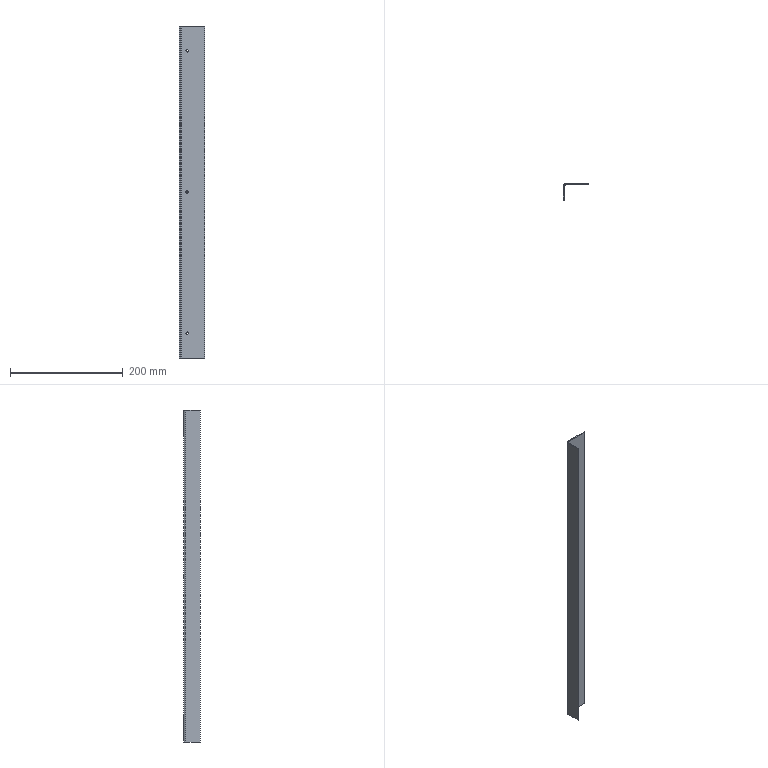Part | STEP file | SYL_0392D6J1SYL0380DJ10-1725835 | 1 solid | 20 faces | box 44.9 x 29.9 x 588 mm | volume 79950 mm3 | plane 12 | cylinder 8 | commonest cylinder face diameters 4.2 x6 4 x1 7.8 x1
STEP:
#1=CARTESIAN_POINT('',(-8.5,29.9,-247.9));
#2=VERTEX_POINT('',#1);
#3=CARTESIAN_POINT('',(-8.5,28.,-247.9));
#4=VERTEX_POINT('',#3);
#5=CARTESIAN_POINT('',(-8.5,28.,-247.9));
#6=DIRECTION('',(0.,-1.,0.));
#7=VECTOR('',#6,1000.);
#8=LINE('',#5,#7);
#9=EDGE_CURVE('',#2,#4,#8,.T.);
#10=ORIENTED_EDGE('',*,*,#9,.F.);
#11=CARTESIAN_POINT('',(-8.5,29.9,-252.1));
#12=VERTEX_POINT('',#11);
#13=CARTESIAN_POINT('',(-8.5,29.9,-250.));
#14=DIRECTION('',(0.,1.,0.));
#15=DIRECTION('',(0.,0.,1.));
#16=AXIS2_PLACEMENT_3D('',#13,#14,#15);
#17=CIRCLE('',#16,2.1);
#18=EDGE_CURVE('',#2,#12,#17,.T.);
#19=ORIENTED_EDGE('',*,*,#18,.T.);
#20=CARTESIAN_POINT('',(-8.5,28.,-252.1));
#21=VERTEX_POINT('',#20);
#22=CARTESIAN_POINT('',(-8.5,28.,-252.1));
#23=DIRECTION('',(0.,-1.,0.));
#24=VECTOR('',#23,1000.);
#25=LINE('',#22,#24);
#26=EDGE_CURVE('',#12,#21,#25,.T.);
#27=ORIENTED_EDGE('',*,*,#26,.T.);
#28=CARTESIAN_POINT('',(-8.5,28.,-250.));
#29=DIRECTION('',(0.,1.,0.));
#30=DIRECTION('',(0.,0.,1.));
#31=AXIS2_PLACEMENT_3D('',#28,#29,#30);
#32=CIRCLE('',#31,2.1);
#33=EDGE_CURVE('',#4,#21,#32,.T.);
#34=ORIENTED_EDGE('',*,*,#33,.F.);
#35=EDGE_LOOP('',(#10,#19,#27,#34));
#36=FACE_OUTER_BOUND('',#35,.T.);
#37=CARTESIAN_POINT('',(-8.5,28.,-250.));
#38=DIRECTION('',(0.,1.,0.));
#39=DIRECTION('',(0.,0.,1.));
#40=AXIS2_PLACEMENT_3D('',#37,#38,#39);
#41=CYLINDRICAL_SURFACE('',#40,2.1);
#42=ADVANCED_FACE('',(#36),#41,.F.);
#43=CARTESIAN_POINT('',(-8.5,29.9,2.1));
#44=VERTEX_POINT('',#43);
#45=CARTESIAN_POINT('',(-8.5,28.,2.1));
#46=VERTEX_POINT('',#45);
#47=CARTESIAN_POINT('',(-8.5,28.,2.1));
#48=DIRECTION('',(0.,-1.,0.));
#49=VECTOR('',#48,1000.);
#50=LINE('',#47,#49);
#51=EDGE_CURVE('',#44,#46,#50,.T.);
#52=ORIENTED_EDGE('',*,*,#51,.F.);
#53=CARTESIAN_POINT('',(-8.5,29.9,-2.1));
#54=VERTEX_POINT('',#53);
#55=CARTESIAN_POINT('',(-8.5,29.9,0.));
#56=DIRECTION('',(0.,1.,0.));
#57=DIRECTION('',(0.,0.,1.));
#58=AXIS2_PLACEMENT_3D('',#55,#56,#57);
#59=CIRCLE('',#58,2.1);
#60=EDGE_CURVE('',#44,#54,#59,.T.);
#61=ORIENTED_EDGE('',*,*,#60,.T.);
#62=CARTESIAN_POINT('',(-8.5,28.,-2.1));
#63=VERTEX_POINT('',#62);
#64=CARTESIAN_POINT('',(-8.5,28.,-2.1));
#65=DIRECTION('',(0.,-1.,0.));
#66=VECTOR('',#65,1000.);
#67=LINE('',#64,#66);
#68=EDGE_CURVE('',#54,#63,#67,.T.);
#69=ORIENTED_EDGE('',*,*,#68,.T.);
#70=CARTESIAN_POINT('',(-8.5,28.,0.));
#71=DIRECTION('',(0.,1.,0.));
#72=DIRECTION('',(0.,0.,1.));
#73=AXIS2_PLACEMENT_3D('',#70,#71,#72);
#74=CIRCLE('',#73,2.1);
#75=EDGE_CURVE('',#46,#63,#74,.T.);
#76=ORIENTED_EDGE('',*,*,#75,.F.);
#77=EDGE_LOOP('',(#52,#61,#69,#76));
#78=FACE_OUTER_BOUND('',#77,.T.);
#79=CARTESIAN_POINT('',(-8.5,28.,0.));
#80=DIRECTION('',(0.,1.,0.));
#81=DIRECTION('',(0.,0.,1.));
#82=AXIS2_PLACEMENT_3D('',#79,#80,#81);
#83=CYLINDRICAL_SURFACE('',#82,2.1);
#84=ADVANCED_FACE('',(#78),#83,.F.);
#85=CARTESIAN_POINT('',(-8.5,29.9,252.1));
#86=VERTEX_POINT('',#85);
#87=CARTESIAN_POINT('',(-8.5,28.,252.1));
#88=VERTEX_POINT('',#87);
#89=CARTESIAN_POINT('',(-8.5,28.,252.1));
#90=DIRECTION('',(0.,-1.,0.));
#91=VECTOR('',#90,1000.);
#92=LINE('',#89,#91);
#93=EDGE_CURVE('',#86,#88,#92,.T.);
#94=ORIENTED_EDGE('',*,*,#93,.F.);
#95=CARTESIAN_POINT('',(-8.5,29.9,247.9));
#96=VERTEX_POINT('',#95);
#97=CARTESIAN_POINT('',(-8.5,29.9,250.));
#98=DIRECTION('',(0.,1.,0.));
#99=DIRECTION('',(0.,0.,1.));
#100=AXIS2_PLACEMENT_3D('',#97,#98,#99);
#101=CIRCLE('',#100,2.1);
#102=EDGE_CURVE('',#86,#96,#101,.T.);
#103=ORIENTED_EDGE('',*,*,#102,.T.);
#104=CARTESIAN_POINT('',(-8.5,28.,247.9));
#105=VERTEX_POINT('',#104);
#106=CARTESIAN_POINT('',(-8.5,28.,247.9));
#107=DIRECTION('',(0.,-1.,0.));
#108=VECTOR('',#107,1000.);
#109=LINE('',#106,#108);
#110=EDGE_CURVE('',#96,#105,#109,.T.);
#111=ORIENTED_EDGE('',*,*,#110,.T.);
#112=CARTESIAN_POINT('',(-8.5,28.,250.));
#113=DIRECTION('',(0.,1.,0.));
#114=DIRECTION('',(0.,0.,1.));
#115=AXIS2_PLACEMENT_3D('',#112,#113,#114);
#116=CIRCLE('',#115,2.1);
#117=EDGE_CURVE('',#88,#105,#116,.T.);
#118=ORIENTED_EDGE('',*,*,#117,.F.);
#119=EDGE_LOOP('',(#94,#103,#111,#118));
#120=FACE_OUTER_BOUND('',#119,.T.);
#121=CARTESIAN_POINT('',(-8.5,28.,250.));
#122=DIRECTION('',(0.,1.,0.));
#123=DIRECTION('',(0.,0.,1.));
#124=AXIS2_PLACEMENT_3D('',#121,#122,#123);
#125=CYLINDRICAL_SURFACE('',#124,2.1);
#126=ADVANCED_FACE('',(#120),#125,.F.);
#127=CARTESIAN_POINT('',(-22.4,0.,294.));
#128=VERTEX_POINT('',#127);
#129=CARTESIAN_POINT('',(-20.5,0.,294.));
#130=VERTEX_POINT('',#129);
#131=CARTESIAN_POINT('',(-20.5,0.,294.));
#132=DIRECTION('',(1.,0.,0.));
#133=VECTOR('',#132,1000.);
#134=LINE('',#131,#133);
#135=EDGE_CURVE('',#128,#130,#134,.T.);
#136=ORIENTED_EDGE('',*,*,#135,.F.);
#137=CARTESIAN_POINT('',(-22.4,0.,-294.));
#138=VERTEX_POINT('',#137);
#139=CARTESIAN_POINT('',(-22.4,0.,-294.));
#140=DIRECTION('',(0.,0.,-1.));
#141=VECTOR('',#140,1000.);
#142=LINE('',#139,#141);
#143=EDGE_CURVE('',#128,#138,#142,.T.);
#144=ORIENTED_EDGE('',*,*,#143,.T.);
#145=CARTESIAN_POINT('',(-20.5,0.,-294.));
#146=VERTEX_POINT('',#145);
#147=CARTESIAN_POINT('',(-20.5,0.,-294.));
#148=DIRECTION('',(1.,0.,0.));
#149=VECTOR('',#148,1000.);
#150=LINE('',#147,#149);
#151=EDGE_CURVE('',#138,#146,#150,.T.);
#152=ORIENTED_EDGE('',*,*,#151,.T.);
#153=CARTESIAN_POINT('',(-20.5,0.,294.));
#154=DIRECTION('',(0.,0.,-1.));
#155=VECTOR('',#154,1000.);
#156=LINE('',#153,#155);
#157=EDGE_CURVE('',#130,#146,#156,.T.);
#158=ORIENTED_EDGE('',*,*,#157,.F.);
#159=EDGE_LOOP('',(#136,#144,#152,#158));
#160=FACE_OUTER_BOUND('',#159,.T.);
#161=CARTESIAN_POINT('',(-20.5,0.,294.));
#162=DIRECTION('',(0.,1.,0.));
#163=DIRECTION('',(0.,0.,-1.));
#164=AXIS2_PLACEMENT_3D('',#161,#162,#163);
#165=PLANE('',#164);
#166=ADVANCED_FACE('',(#160),#165,.F.);
#167=ORIENTED_EDGE('',*,*,#151,.F.);
#168=CARTESIAN_POINT('',(-22.4,26.,-294.));
#169=VERTEX_POINT('',#168);
#170=CARTESIAN_POINT('',(-22.4,30.,-294.));
#171=DIRECTION('',(0.,1.,0.));
#172=VECTOR('',#171,1000.);
#173=LINE('',#170,#172);
#174=EDGE_CURVE('',#138,#169,#173,.T.);
#175=ORIENTED_EDGE('',*,*,#174,.T.);
#176=CARTESIAN_POINT('',(-20.5,26.,-294.));
#177=VERTEX_POINT('',#176);
#178=CARTESIAN_POINT('',(-20.5,26.,-294.));
#179=DIRECTION('',(1.,0.,0.));
#180=VECTOR('',#179,1000.);
#181=LINE('',#178,#180);
#182=EDGE_CURVE('',#169,#177,#181,.T.);
#183=ORIENTED_EDGE('',*,*,#182,.T.);
#184=CARTESIAN_POINT('',(-20.5,0.,-294.));
#185=DIRECTION('',(0.,1.,0.));
#186=VECTOR('',#185,1000.);
#187=LINE('',#184,#186);
#188=EDGE_CURVE('',#146,#177,#187,.T.);
#189=ORIENTED_EDGE('',*,*,#188,.F.);
#190=EDGE_LOOP('',(#167,#175,#183,#189));
#191=FACE_OUTER_BOUND('',#190,.T.);
#192=CARTESIAN_POINT('',(-20.5,0.,-294.));
#193=DIRECTION('',(0.,0.,1.));
#194=DIRECTION('',(0.,1.,0.));
#195=AXIS2_PLACEMENT_3D('',#192,#193,#194);
#196=PLANE('',#195);
#197=ADVANCED_FACE('',(#191),#196,.F.);
#198=ORIENTED_EDGE('',*,*,#182,.F.);
#199=CARTESIAN_POINT('',(-18.5,29.9,-294.));
#200=VERTEX_POINT('',#199);
#201=CARTESIAN_POINT('',(-18.5,26.,-294.));
#202=DIRECTION('',(0.,0.,1.));
#203=DIRECTION('',(-1.,0.,0.));
#204=AXIS2_PLACEMENT_3D('',#201,#202,#203);
#205=CIRCLE('',#204,3.9);
#206=EDGE_CURVE('',#200,#169,#205,.T.);
#207=ORIENTED_EDGE('',*,*,#206,.F.);
#208=CARTESIAN_POINT('',(-18.5,28.,-294.));
#209=VERTEX_POINT('',#208);
#210=CARTESIAN_POINT('',(-18.5,28.,-294.));
#211=DIRECTION('',(0.,-1.,0.));
#212=VECTOR('',#211,1000.);
#213=LINE('',#210,#212);
#214=EDGE_CURVE('',#200,#209,#213,.T.);
#215=ORIENTED_EDGE('',*,*,#214,.T.);
#216=CARTESIAN_POINT('',(-18.5,26.,-294.));
#217=DIRECTION('',(0.,0.,1.));
#218=DIRECTION('',(0.,1.,0.));
#219=AXIS2_PLACEMENT_3D('',#216,#217,#218);
#220=CIRCLE('',#219,2.);
#221=EDGE_CURVE('',#209,#177,#220,.T.);
#222=ORIENTED_EDGE('',*,*,#221,.T.);
#223=EDGE_LOOP('',(#198,#207,#215,#222));
#224=FACE_OUTER_BOUND('',#223,.T.);
#225=CARTESIAN_POINT('',(-18.5,26.,-294.));
#226=DIRECTION('',(0.,0.,-1.));
#227=DIRECTION('',(-1.,0.,0.));
#228=AXIS2_PLACEMENT_3D('',#225,#226,#227);
#229=PLANE('',#228);
#230=ADVANCED_FACE('',(#224),#229,.T.);
#231=ORIENTED_EDGE('',*,*,#214,.F.);
#232=CARTESIAN_POINT('',(22.5,29.9,-294.));
#233=VERTEX_POINT('',#232);
#234=CARTESIAN_POINT('',(22.5,29.9,-294.));
#235=DIRECTION('',(1.,0.,0.));
#236=VECTOR('',#235,1000.);
#237=LINE('',#234,#236);
#238=EDGE_CURVE('',#200,#233,#237,.T.);
#239=ORIENTED_EDGE('',*,*,#238,.T.);
#240=CARTESIAN_POINT('',(22.5,28.,-294.));
#241=VERTEX_POINT('',#240);
#242=CARTESIAN_POINT('',(22.5,28.,-294.));
#243=DIRECTION('',(0.,-1.,0.));
#244=VECTOR('',#243,1000.);
#245=LINE('',#242,#244);
#246=EDGE_CURVE('',#233,#241,#245,.T.);
#247=ORIENTED_EDGE('',*,*,#246,.T.);
#248=CARTESIAN_POINT('',(-18.5,28.,-294.));
#249=DIRECTION('',(1.,0.,0.));
#250=VECTOR('',#249,1000.);
#251=LINE('',#248,#250);
#252=EDGE_CURVE('',#209,#241,#251,.T.);
#253=ORIENTED_EDGE('',*,*,#252,.F.);
#254=EDGE_LOOP('',(#231,#239,#247,#253));
#255=FACE_OUTER_BOUND('',#254,.T.);
#256=CARTESIAN_POINT('',(-18.5,28.,-294.));
#257=DIRECTION('',(0.,0.,1.));
#258=DIRECTION('',(1.,0.,0.));
#259=AXIS2_PLACEMENT_3D('',#256,#257,#258);
#260=PLANE('',#259);
#261=ADVANCED_FACE('',(#255),#260,.F.);
#262=ORIENTED_EDGE('',*,*,#246,.F.);
#263=CARTESIAN_POINT('',(22.5,29.9,294.));
#264=VERTEX_POINT('',#263);
#265=CARTESIAN_POINT('',(22.5,29.9,-294.));
#266=DIRECTION('',(0.,0.,1.));
#267=VECTOR('',#266,1000.);
#268=LINE('',#265,#267);
#269=EDGE_CURVE('',#233,#264,#268,.T.);
#270=ORIENTED_EDGE('',*,*,#269,.T.);
#271=CARTESIAN_POINT('',(22.5,28.,294.));
#272=VERTEX_POINT('',#271);
#273=CARTESIAN_POINT('',(22.5,28.,294.));
#274=DIRECTION('',(0.,-1.,0.));
#275=VECTOR('',#274,1000.);
#276=LINE('',#273,#275);
#277=EDGE_CURVE('',#264,#272,#276,.T.);
#278=ORIENTED_EDGE('',*,*,#277,.T.);
#279=CARTESIAN_POINT('',(22.5,28.,-294.));
#280=DIRECTION('',(0.,0.,1.));
#281=VECTOR('',#280,1000.);
#282=LINE('',#279,#281);
#283=EDGE_CURVE('',#241,#272,#282,.T.);
#284=ORIENTED_EDGE('',*,*,#283,.F.);
#285=EDGE_LOOP('',(#262,#270,#278,#284));
#286=FACE_OUTER_BOUND('',#285,.T.);
#287=CARTESIAN_POINT('',(22.5,28.,-294.));
#288=DIRECTION('',(-1.,0.,0.));
#289=DIRECTION('',(0.,0.,1.));
#290=AXIS2_PLACEMENT_3D('',#287,#288,#289);
#291=PLANE('',#290);
#292=ADVANCED_FACE('',(#286),#291,.F.);
#293=ORIENTED_EDGE('',*,*,#277,.F.);
#294=CARTESIAN_POINT('',(-18.5,29.9,294.));
#295=VERTEX_POINT('',#294);
#296=CARTESIAN_POINT('',(22.5,29.9,294.));
#297=DIRECTION('',(-1.,0.,0.));
#298=VECTOR('',#297,1000.);
#299=LINE('',#296,#298);
#300=EDGE_CURVE('',#264,#295,#299,.T.);
#301=ORIENTED_EDGE('',*,*,#300,.T.);
#302=CARTESIAN_POINT('',(-18.5,28.,294.));
#303=VERTEX_POINT('',#302);
#304=CARTESIAN_POINT('',(-18.5,28.,294.));
#305=DIRECTION('',(0.,-1.,0.));
#306=VECTOR('',#305,1000.);
#307=LINE('',#304,#306);
#308=EDGE_CURVE('',#295,#303,#307,.T.);
#309=ORIENTED_EDGE('',*,*,#308,.T.);
#310=CARTESIAN_POINT('',(22.5,28.,294.));
#311=DIRECTION('',(-1.,0.,0.));
#312=VECTOR('',#311,1000.);
#313=LINE('',#310,#312);
#314=EDGE_CURVE('',#272,#303,#313,.T.);
#315=ORIENTED_EDGE('',*,*,#314,.F.);
#316=EDGE_LOOP('',(#293,#301,#309,#315));
#317=FACE_OUTER_BOUND('',#316,.T.);
#318=CARTESIAN_POINT('',(22.5,28.,294.));
#319=DIRECTION('',(0.,0.,-1.));
#320=DIRECTION('',(-1.,0.,0.));
#321=AXIS2_PLACEMENT_3D('',#318,#319,#320);
#322=PLANE('',#321);
#323=ADVANCED_FACE('',(#317),#322,.F.);
#324=ORIENTED_EDGE('',*,*,#308,.F.);
#325=CARTESIAN_POINT('',(-22.4,26.,294.));
#326=VERTEX_POINT('',#325);
#327=CARTESIAN_POINT('',(-18.5,26.,294.));
#328=DIRECTION('',(0.,0.,-1.));
#329=DIRECTION('',(-1.,0.,0.));
#330=AXIS2_PLACEMENT_3D('',#327,#328,#329);
#331=CIRCLE('',#330,3.9);
#332=EDGE_CURVE('',#326,#295,#331,.T.);
#333=ORIENTED_EDGE('',*,*,#332,.F.);
#334=CARTESIAN_POINT('',(-20.5,26.,294.));
#335=VERTEX_POINT('',#334);
#336=CARTESIAN_POINT('',(-20.5,26.,294.));
#337=DIRECTION('',(1.,0.,0.));
#338=VECTOR('',#337,1000.);
#339=LINE('',#336,#338);
#340=EDGE_CURVE('',#326,#335,#339,.T.);
#341=ORIENTED_EDGE('',*,*,#340,.T.);
#342=CARTESIAN_POINT('',(-18.5,26.,294.));
#343=DIRECTION('',(0.,0.,-1.));
#344=DIRECTION('',(-1.,0.,0.));
#345=AXIS2_PLACEMENT_3D('',#342,#343,#344);
#346=CIRCLE('',#345,2.);
#347=EDGE_CURVE('',#335,#303,#346,.T.);
#348=ORIENTED_EDGE('',*,*,#347,.T.);
#349=EDGE_LOOP('',(#324,#333,#341,#348));
#350=FACE_OUTER_BOUND('',#349,.T.);
#351=CARTESIAN_POINT('',(-18.5,26.,294.));
#352=DIRECTION('',(0.,0.,1.));
#353=DIRECTION('',(1.,0.,0.));
#354=AXIS2_PLACEMENT_3D('',#351,#352,#353);
#355=PLANE('',#354);
#356=ADVANCED_FACE('',(#350),#355,.T.);
#357=CARTESIAN_POINT('',(-8.5,29.9,250.));
#358=DIRECTION('',(0.,1.,0.));
#359=DIRECTION('',(0.,0.,1.));
#360=AXIS2_PLACEMENT_3D('',#357,#358,#359);
#361=CIRCLE('',#360,2.1);
#362=EDGE_CURVE('',#96,#86,#361,.T.);
#363=ORIENTED_EDGE('',*,*,#362,.T.);
#364=ORIENTED_EDGE('',*,*,#93,.T.);
#365=CARTESIAN_POINT('',(-8.5,28.,250.));
#366=DIRECTION('',(0.,1.,0.));
#367=DIRECTION('',(0.,0.,-1.));
#368=AXIS2_PLACEMENT_3D('',#365,#366,#367);
#369=CIRCLE('',#368,2.1);
#370=EDGE_CURVE('',#105,#88,#369,.T.);
#371=ORIENTED_EDGE('',*,*,#370,.F.);
#372=ORIENTED_EDGE('',*,*,#110,.F.);
#373=EDGE_LOOP('',(#363,#364,#371,#372));
#374=FACE_OUTER_BOUND('',#373,.T.);
#375=CARTESIAN_POINT('',(-8.5,28.,250.));
#376=DIRECTION('',(0.,1.,0.));
#377=DIRECTION('',(0.,0.,1.));
#378=AXIS2_PLACEMENT_3D('',#375,#376,#377);
#379=CYLINDRICAL_SURFACE('',#378,2.1);
#380=ADVANCED_FACE('',(#374),#379,.F.);
#381=CARTESIAN_POINT('',(-8.5,29.9,0.));
#382=DIRECTION('',(0.,1.,0.));
#383=DIRECTION('',(0.,0.,1.));
#384=AXIS2_PLACEMENT_3D('',#381,#382,#383);
#385=CIRCLE('',#384,2.1);
#386=EDGE_CURVE('',#54,#44,#385,.T.);
#387=ORIENTED_EDGE('',*,*,#386,.T.);
#388=ORIENTED_EDGE('',*,*,#51,.T.);
#389=CARTESIAN_POINT('',(-8.5,28.,0.));
#390=DIRECTION('',(0.,1.,0.));
#391=DIRECTION('',(0.,0.,-1.));
#392=AXIS2_PLACEMENT_3D('',#389,#390,#391);
#393=CIRCLE('',#392,2.1);
#394=EDGE_CURVE('',#63,#46,#393,.T.);
#395=ORIENTED_EDGE('',*,*,#394,.F.);
#396=ORIENTED_EDGE('',*,*,#68,.F.);
#397=EDGE_LOOP('',(#387,#388,#395,#396));
#398=FACE_OUTER_BOUND('',#397,.T.);
#399=CARTESIAN_POINT('',(-8.5,28.,0.));
#400=DIRECTION('',(0.,1.,0.));
#401=DIRECTION('',(0.,0.,1.));
#402=AXIS2_PLACEMENT_3D('',#399,#400,#401);
#403=CYLINDRICAL_SURFACE('',#402,2.1);
#404=ADVANCED_FACE('',(#398),#403,.F.);
#405=CARTESIAN_POINT('',(-8.5,29.9,-250.));
#406=DIRECTION('',(0.,1.,0.));
#407=DIRECTION('',(0.,0.,1.));
#408=AXIS2_PLACEMENT_3D('',#405,#406,#407);
#409=CIRCLE('',#408,2.1);
#410=EDGE_CURVE('',#12,#2,#409,.T.);
#411=ORIENTED_EDGE('',*,*,#410,.T.);
#412=ORIENTED_EDGE('',*,*,#9,.T.);
#413=CARTESIAN_POINT('',(-8.5,28.,-250.));
#414=DIRECTION('',(0.,1.,0.));
#415=DIRECTION('',(0.,0.,-1.));
#416=AXIS2_PLACEMENT_3D('',#413,#414,#415);
#417=CIRCLE('',#416,2.1);
#418=EDGE_CURVE('',#21,#4,#417,.T.);
#419=ORIENTED_EDGE('',*,*,#418,.F.);
#420=ORIENTED_EDGE('',*,*,#26,.F.);
#421=EDGE_LOOP('',(#411,#412,#419,#420));
#422=FACE_OUTER_BOUND('',#421,.T.);
#423=CARTESIAN_POINT('',(-8.5,28.,-250.));
#424=DIRECTION('',(0.,1.,0.));
#425=DIRECTION('',(0.,0.,1.));
#426=AXIS2_PLACEMENT_3D('',#423,#424,#425);
#427=CYLINDRICAL_SURFACE('',#426,2.1);
#428=ADVANCED_FACE('',(#422),#427,.F.);
#429=CARTESIAN_POINT('',(-22.4,30.,294.));
#430=DIRECTION('',(0.,-1.,0.));
#431=VECTOR('',#430,1000.);
#432=LINE('',#429,#431);
#433=EDGE_CURVE('',#326,#128,#432,.T.);
#434=ORIENTED_EDGE('',*,*,#433,.T.);
#435=ORIENTED_EDGE('',*,*,#135,.T.);
#436=CARTESIAN_POINT('',(-20.5,26.,294.));
#437=DIRECTION('',(0.,-1.,0.));
#438=VECTOR('',#437,1000.);
#439=LINE('',#436,#438);
#440=EDGE_CURVE('',#335,#130,#439,.T.);
#441=ORIENTED_EDGE('',*,*,#440,.F.);
#442=ORIENTED_EDGE('',*,*,#340,.F.);
#443=EDGE_LOOP('',(#434,#435,#441,#442));
#444=FACE_OUTER_BOUND('',#443,.T.);
#445=CARTESIAN_POINT('',(-20.5,26.,294.));
#446=DIRECTION('',(0.,0.,-1.));
#447=DIRECTION('',(0.,-1.,0.));
#448=AXIS2_PLACEMENT_3D('',#445,#446,#447);
#449=PLANE('',#448);
#450=ADVANCED_FACE('',(#444),#449,.F.);
#451=ORIENTED_EDGE('',*,*,#347,.F.);
#452=CARTESIAN_POINT('',(-20.5,26.,294.));
#453=DIRECTION('',(0.,0.,-1.));
#454=VECTOR('',#453,1000.);
#455=LINE('',#452,#454);
#456=EDGE_CURVE('',#335,#177,#455,.T.);
#457=ORIENTED_EDGE('',*,*,#456,.T.);
#458=ORIENTED_EDGE('',*,*,#221,.F.);
#459=CARTESIAN_POINT('',(-18.5,28.,-294.));
#460=DIRECTION('',(0.,0.,1.));
#461=VECTOR('',#460,1000.);
#462=LINE('',#459,#461);
#463=EDGE_CURVE('',#209,#303,#462,.T.);
#464=ORIENTED_EDGE('',*,*,#463,.T.);
#465=EDGE_LOOP('',(#451,#457,#458,#464));
#466=FACE_OUTER_BOUND('',#465,.T.);
#467=CARTESIAN_POINT('',(-18.5,26.,-294.));
#468=DIRECTION('',(0.,0.,-1.));
#469=DIRECTION('',(-1.,0.,0.));
#470=AXIS2_PLACEMENT_3D('',#467,#468,#469);
#471=CYLINDRICAL_SURFACE('',#470,2.);
#472=ADVANCED_FACE('',(#466),#471,.F.);
#473=ORIENTED_EDGE('',*,*,#117,.T.);
#474=ORIENTED_EDGE('',*,*,#370,.T.);
#475=EDGE_LOOP('',(#473,#474));
#476=FACE_BOUND('',#475,.T.);
#477=ORIENTED_EDGE('',*,*,#75,.T.);
#478=ORIENTED_EDGE('',*,*,#394,.T.);
#479=EDGE_LOOP('',(#477,#478));
#480=FACE_BOUND('',#479,.T.);
#481=ORIENTED_EDGE('',*,*,#33,.T.);
#482=ORIENTED_EDGE('',*,*,#418,.T.);
#483=EDGE_LOOP('',(#481,#482));
#484=FACE_BOUND('',#483,.T.);
#485=ORIENTED_EDGE('',*,*,#463,.F.);
#486=ORIENTED_EDGE('',*,*,#252,.T.);
#487=ORIENTED_EDGE('',*,*,#283,.T.);
#488=ORIENTED_EDGE('',*,*,#314,.T.);
#489=EDGE_LOOP('',(#485,#486,#487,#488));
#490=FACE_OUTER_BOUND('',#489,.T.);
#491=CARTESIAN_POINT('',(22.5,28.,-294.));
#492=DIRECTION('',(0.,1.,0.));
#493=DIRECTION('',(1.,0.,0.));
#494=AXIS2_PLACEMENT_3D('',#491,#492,#493);
#495=PLANE('',#494);
#496=ADVANCED_FACE('',(#476,#480,#484,#490),#495,.F.);
#497=ORIENTED_EDGE('',*,*,#157,.T.);
#498=ORIENTED_EDGE('',*,*,#188,.T.);
#499=ORIENTED_EDGE('',*,*,#456,.F.);
#500=ORIENTED_EDGE('',*,*,#440,.T.);
#501=EDGE_LOOP('',(#497,#498,#499,#500));
#502=FACE_OUTER_BOUND('',#501,.T.);
#503=CARTESIAN_POINT('',(-20.5,30.,-294.));
#504=DIRECTION('',(-1.,0.,0.));
#505=DIRECTION('',(0.,0.,1.));
#506=AXIS2_PLACEMENT_3D('',#503,#504,#505);
#507=PLANE('',#506);
#508=ADVANCED_FACE('',(#502),#507,.F.);
#509=ORIENTED_EDGE('',*,*,#332,.T.);
#510=CARTESIAN_POINT('',(-18.5,29.9,-294.));
#511=DIRECTION('',(0.,0.,1.));
#512=VECTOR('',#511,1000.);
#513=LINE('',#510,#512);
#514=EDGE_CURVE('',#200,#295,#513,.T.);
#515=ORIENTED_EDGE('',*,*,#514,.F.);
#516=ORIENTED_EDGE('',*,*,#206,.T.);
#517=CARTESIAN_POINT('',(-22.4,26.,-294.));
#518=DIRECTION('',(0.,0.,-1.));
#519=VECTOR('',#518,1000.);
#520=LINE('',#517,#519);
#521=EDGE_CURVE('',#326,#169,#520,.T.);
#522=ORIENTED_EDGE('',*,*,#521,.F.);
#523=EDGE_LOOP('',(#509,#515,#516,#522));
#524=FACE_OUTER_BOUND('',#523,.T.);
#525=CARTESIAN_POINT('',(-18.5,26.,-294.));
#526=DIRECTION('',(0.,0.,-1.));
#527=DIRECTION('',(-1.,0.,0.));
#528=AXIS2_PLACEMENT_3D('',#525,#526,#527);
#529=CYLINDRICAL_SURFACE('',#528,3.9);
#530=ADVANCED_FACE('',(#524),#529,.T.);
#531=ORIENTED_EDGE('',*,*,#102,.F.);
#532=ORIENTED_EDGE('',*,*,#362,.F.);
#533=EDGE_LOOP('',(#531,#532));
#534=FACE_BOUND('',#533,.T.);
#535=ORIENTED_EDGE('',*,*,#60,.F.);
#536=ORIENTED_EDGE('',*,*,#386,.F.);
#537=EDGE_LOOP('',(#535,#536));
#538=FACE_BOUND('',#537,.T.);
#539=ORIENTED_EDGE('',*,*,#18,.F.);
#540=ORIENTED_EDGE('',*,*,#410,.F.);
#541=EDGE_LOOP('',(#539,#540));
#542=FACE_BOUND('',#541,.T.);
#543=ORIENTED_EDGE('',*,*,#514,.T.);
#544=ORIENTED_EDGE('',*,*,#300,.F.);
#545=ORIENTED_EDGE('',*,*,#269,.F.);
#546=ORIENTED_EDGE('',*,*,#238,.F.);
#547=EDGE_LOOP('',(#543,#544,#545,#546));
#548=FACE_OUTER_BOUND('',#547,.T.);
#549=CARTESIAN_POINT('',(22.5,29.9,-294.));
#550=DIRECTION('',(0.,1.,0.));
#551=DIRECTION('',(1.,0.,0.));
#552=AXIS2_PLACEMENT_3D('',#549,#550,#551);
#553=PLANE('',#552);
#554=ADVANCED_FACE('',(#534,#538,#542,#548),#553,.T.);
#555=ORIENTED_EDGE('',*,*,#143,.F.);
#556=ORIENTED_EDGE('',*,*,#433,.F.);
#557=ORIENTED_EDGE('',*,*,#521,.T.);
#558=ORIENTED_EDGE('',*,*,#174,.F.);
#559=EDGE_LOOP('',(#555,#556,#557,#558));
#560=FACE_OUTER_BOUND('',#559,.T.);
#561=CARTESIAN_POINT('',(-22.4,30.,-294.));
#562=DIRECTION('',(-1.,0.,0.));
#563=DIRECTION('',(0.,0.,1.));
#564=AXIS2_PLACEMENT_3D('',#561,#562,#563);
#565=PLANE('',#564);
#566=ADVANCED_FACE('',(#560),#565,.T.);
#567=CLOSED_SHELL('',(#42,#84,#126,#166,#197,#230,#261,#292,#323,#356,#380,#404,#428,#450,#472,#496,#508,#530,#554,#566));
#568=MANIFOLD_SOLID_BREP('',#567);
#569=CARTESIAN_POINT('',(0.,0.,0.));
#570=DIRECTION('',(0.,0.,1.));
#571=DIRECTION('',(1.,0.,0.));
#572=AXIS2_PLACEMENT_3D('',#569,#570,#571);
#573=(LENGTH_UNIT()NAMED_UNIT(*)SI_UNIT(.MILLI.,.METRE.));
#574=UNCERTAINTY_MEASURE_WITH_UNIT(LENGTH_MEASURE(0.00001),#573,'','');
#575=(NAMED_UNIT(*)PLANE_ANGLE_UNIT()SI_UNIT($,.RADIAN.));
#576=(NAMED_UNIT(*)SI_UNIT($,.STERADIAN.)SOLID_ANGLE_UNIT());
#577=(GEOMETRIC_REPRESENTATION_CONTEXT(3)GLOBAL_UNCERTAINTY_ASSIGNED_CONTEXT((#574))GLOBAL_UNIT_ASSIGNED_CONTEXT((#573,#575,#576))REPRESENTATION_CONTEXT('',''));
#578=ADVANCED_BREP_SHAPE_REPRESENTATION('',(#568,#572),#577);